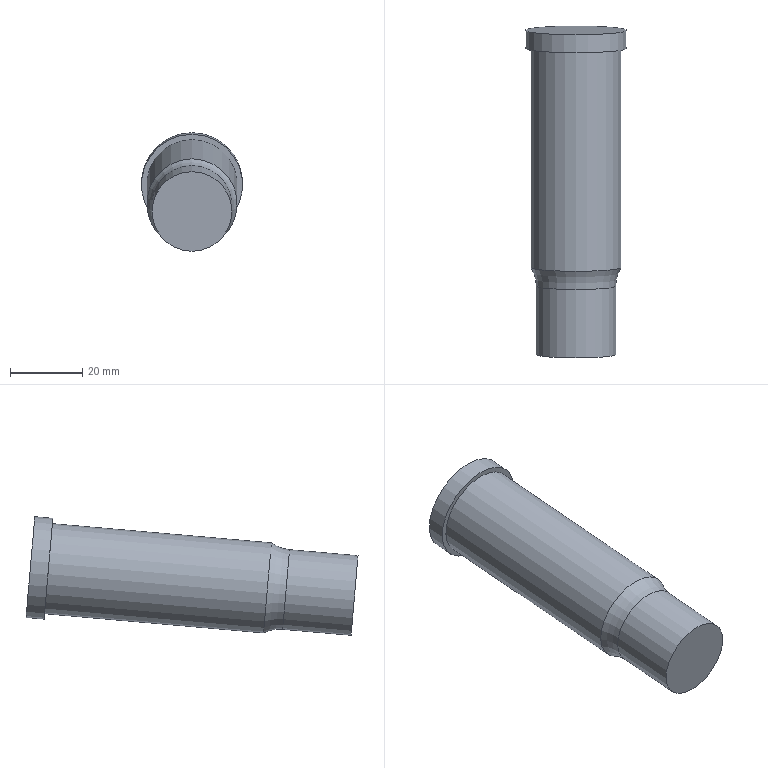Part | NX | features SPAS 25-80-22.10 2 | 1 solid | 7 faces | box 28 x 91.841 x 32.799 mm | volume 42384 mm3 | plane 3 | cylinder 3 | torus 1 | commonest cylinder face diameters 22.1 x1 25 x1 28 x1
STEP:
#1=CARTESIAN_POINT('',(-150.187,51.383,-27.306));
#2=VERTEX_POINT('',#1);
#3=CARTESIAN_POINT('',(-150.187,52.346,-38.314));
#4=DIRECTION('',(0.,0.9962,0.08716));
#5=DIRECTION('',(0.,-0.08716,0.9962));
#6=AXIS2_PLACEMENT_3D('',#3,#4,#5);
#7=CIRCLE('',#6,11.05);
#8=EDGE_CURVE('',#2,#2,#7,.T.);
#9=ORIENTED_EDGE('',*,*,#8,.F.);
#10=EDGE_LOOP('',(#9));
#11=FACE_BOUND('',#10,.T.);
#12=CARTESIAN_POINT('',(-150.187,52.346,-38.314));
#13=DIRECTION('',(0.,-0.9962,-0.08716));
#14=DIRECTION('',(0.,0.08716,-0.9962));
#15=AXIS2_PLACEMENT_3D('',#12,#13,#14);
#16=PLANE('',#15);
#17=ADVANCED_FACE('',(#11),#16,.T.);
#18=CARTESIAN_POINT('',(-150.187,70.311,-25.65));
#19=VERTEX_POINT('',#18);
#20=CARTESIAN_POINT('',(-150.187,71.274,-36.658));
#21=DIRECTION('',(0.,0.9962,0.08716));
#22=DIRECTION('',(0.,-0.08716,0.9962));
#23=AXIS2_PLACEMENT_3D('',#20,#21,#22);
#24=CIRCLE('',#23,11.05);
#25=EDGE_CURVE('',#19,#19,#24,.F.);
#26=ORIENTED_EDGE('',*,*,#25,.T.);
#27=EDGE_LOOP('',(#26));
#28=FACE_BOUND('',#27,.T.);
#29=ORIENTED_EDGE('',*,*,#8,.T.);
#30=EDGE_LOOP('',(#29));
#31=FACE_BOUND('',#30,.T.);
#32=CARTESIAN_POINT('',(-150.187,52.346,-38.314));
#33=DIRECTION('',(0.,0.9962,0.08716));
#34=DIRECTION('',(0.,-0.08716,0.9962));
#35=AXIS2_PLACEMENT_3D('',#32,#33,#34);
#36=CYLINDRICAL_SURFACE('',#35,11.05);
#37=ADVANCED_FACE('',(#28,#31),#36,.T.);
#38=CARTESIAN_POINT('',(-150.187,138.112,-43.358));
#39=VERTEX_POINT('',#38);
#40=CARTESIAN_POINT('',(-150.187,137.023,-30.905));
#41=DIRECTION('',(0.,-0.9962,-0.08716));
#42=DIRECTION('',(0.,0.08716,-0.9962));
#43=AXIS2_PLACEMENT_3D('',#40,#41,#42);
#44=CIRCLE('',#43,12.5);
#45=EDGE_CURVE('',#39,#39,#44,.F.);
#46=ORIENTED_EDGE('',*,*,#45,.F.);
#47=EDGE_LOOP('',(#46));
#48=FACE_BOUND('',#47,.T.);
#49=CARTESIAN_POINT('',(-150.187,75.351,-23.753));
#50=VERTEX_POINT('',#49);
#51=CARTESIAN_POINT('',(-150.187,76.441,-36.206));
#52=DIRECTION('',(0.,0.9962,0.08716));
#53=DIRECTION('',(0.,-0.08716,0.9962));
#54=AXIS2_PLACEMENT_3D('',#51,#52,#53);
#55=CIRCLE('',#54,12.5);
#56=EDGE_CURVE('',#50,#50,#55,.T.);
#57=ORIENTED_EDGE('',*,*,#56,.T.);
#58=EDGE_LOOP('',(#57));
#59=FACE_BOUND('',#58,.T.);
#60=CARTESIAN_POINT('',(-150.187,76.441,-36.206));
#61=DIRECTION('',(0.,0.9962,0.08716));
#62=DIRECTION('',(0.,-0.08716,0.9962));
#63=AXIS2_PLACEMENT_3D('',#60,#61,#62);
#64=CYLINDRICAL_SURFACE('',#63,12.5);
#65=ADVANCED_FACE('',(#48,#59),#64,.T.);
#66=CARTESIAN_POINT('',(-150.187,140.784,-16.523));
#67=VERTEX_POINT('',#66);
#68=CARTESIAN_POINT('',(-150.187,142.004,-30.47));
#69=DIRECTION('',(0.,0.9962,0.08716));
#70=DIRECTION('',(0.,-0.08716,0.9962));
#71=AXIS2_PLACEMENT_3D('',#68,#69,#70);
#72=CIRCLE('',#71,14.);
#73=EDGE_CURVE('',#67,#67,#72,.F.);
#74=ORIENTED_EDGE('',*,*,#73,.F.);
#75=EDGE_LOOP('',(#74));
#76=FACE_BOUND('',#75,.T.);
#77=CARTESIAN_POINT('',(-150.187,142.004,-30.47));
#78=DIRECTION('',(0.,0.9962,0.08716));
#79=DIRECTION('',(0.,-0.08716,0.9962));
#80=AXIS2_PLACEMENT_3D('',#77,#78,#79);
#81=PLANE('',#80);
#82=ADVANCED_FACE('',(#76),#81,.T.);
#83=ORIENTED_EDGE('',*,*,#45,.T.);
#84=EDGE_LOOP('',(#83));
#85=FACE_BOUND('',#84,.T.);
#86=CARTESIAN_POINT('',(-150.187,138.243,-44.852));
#87=VERTEX_POINT('',#86);
#88=CARTESIAN_POINT('',(-150.187,137.023,-30.905));
#89=DIRECTION('',(0.,-0.9962,-0.08716));
#90=DIRECTION('',(0.,0.08716,-0.9962));
#91=AXIS2_PLACEMENT_3D('',#88,#89,#90);
#92=CIRCLE('',#91,14.);
#93=EDGE_CURVE('',#87,#87,#92,.F.);
#94=ORIENTED_EDGE('',*,*,#93,.F.);
#95=EDGE_LOOP('',(#94));
#96=FACE_BOUND('',#95,.T.);
#97=CARTESIAN_POINT('',(-150.187,137.023,-30.905));
#98=DIRECTION('',(0.,-0.9962,-0.08716));
#99=DIRECTION('',(0.,0.08716,-0.9962));
#100=AXIS2_PLACEMENT_3D('',#97,#98,#99);
#101=PLANE('',#100);
#102=ADVANCED_FACE('',(#85,#96),#101,.T.);
#103=ORIENTED_EDGE('',*,*,#73,.T.);
#104=EDGE_LOOP('',(#103));
#105=FACE_BOUND('',#104,.T.);
#106=ORIENTED_EDGE('',*,*,#93,.T.);
#107=EDGE_LOOP('',(#106));
#108=FACE_BOUND('',#107,.T.);
#109=CARTESIAN_POINT('',(-150.187,127.061,-31.777));
#110=DIRECTION('',(0.,0.9962,0.08716));
#111=DIRECTION('',(0.,-0.08716,0.9962));
#112=AXIS2_PLACEMENT_3D('',#109,#110,#111);
#113=CYLINDRICAL_SURFACE('',#112,14.);
#114=ADVANCED_FACE('',(#105,#108),#113,.T.);
#115=ORIENTED_EDGE('',*,*,#25,.F.);
#116=EDGE_LOOP('',(#115));
#117=FACE_BOUND('',#116,.T.);
#118=ORIENTED_EDGE('',*,*,#56,.F.);
#119=EDGE_LOOP('',(#118));
#120=FACE_BOUND('',#119,.T.);
#121=CARTESIAN_POINT('',(-150.187,71.274,-36.658));
#122=DIRECTION('',(0.,0.9962,0.08716));
#123=DIRECTION('',(0.,-0.08716,0.9962));
#124=AXIS2_PLACEMENT_3D('',#121,#122,#123);
#125=TOROIDAL_SURFACE('',#124,21.05,10.);
#126=ADVANCED_FACE('',(#117,#120),#125,.F.);
#127=CLOSED_SHELL('',(#17,#37,#65,#82,#102,#114,#126));
#128=MANIFOLD_SOLID_BREP('',#127);
#129=(LENGTH_UNIT()NAMED_UNIT(*)SI_UNIT(.MILLI.,.METRE.));
#130=UNCERTAINTY_MEASURE_WITH_UNIT(LENGTH_MEASURE(0.00001),#129,'','');
#131=(NAMED_UNIT(*)PLANE_ANGLE_UNIT()SI_UNIT($,.RADIAN.));
#132=(NAMED_UNIT(*)SI_UNIT($,.STERADIAN.)SOLID_ANGLE_UNIT());
#133=(GEOMETRIC_REPRESENTATION_CONTEXT(3)GLOBAL_UNCERTAINTY_ASSIGNED_CONTEXT((#130))GLOBAL_UNIT_ASSIGNED_CONTEXT((#129,#131,#132))REPRESENTATION_CONTEXT('',''));
#134=ADVANCED_BREP_SHAPE_REPRESENTATION('',(#128),#133);